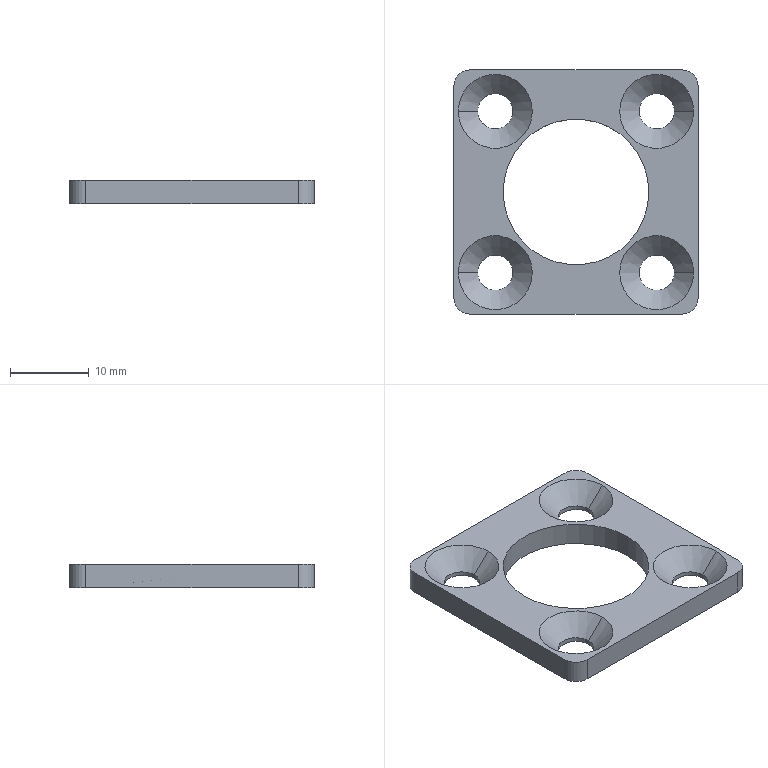Part | NX | features BREP 1 | 1 solid | 28 faces | box 31 x 31 x 3 mm | volume 1644 mm3 | cylinder 14 | cone 8 | plane 6 | commonest cylinder face diameters 4.5 x8 4 x4 18.5 x2
STEP:
#1=CARTESIAN_POINT('',(5.55,10.25,3.));
#2=VERTEX_POINT('',#1);
#3=CARTESIAN_POINT('',(8.,10.25,0.55));
#4=VERTEX_POINT('',#3);
#5=CARTESIAN_POINT('',(5.55,10.25,3.));
#6=DIRECTION('',(-0.7071,0.,0.7071));
#7=VECTOR('',#6,1000.);
#8=LINE('',#5,#7);
#9=EDGE_CURVE('',#2,#4,#8,.F.);
#10=ORIENTED_EDGE('',*,*,#9,.T.);
#11=CARTESIAN_POINT('',(12.5,10.25,0.55));
#12=VERTEX_POINT('',#11);
#13=CARTESIAN_POINT('',(10.25,10.25,0.55));
#14=DIRECTION('',(0.,0.,1.));
#15=DIRECTION('',(1.,0.,0.));
#16=AXIS2_PLACEMENT_3D('',#13,#14,#15);
#17=CIRCLE('',#16,2.25);
#18=EDGE_CURVE('',#12,#4,#17,.T.);
#19=ORIENTED_EDGE('',*,*,#18,.F.);
#20=CARTESIAN_POINT('',(14.95,10.25,3.));
#21=VERTEX_POINT('',#20);
#22=CARTESIAN_POINT('',(14.95,10.25,3.));
#23=DIRECTION('',(0.7071,0.,0.7071));
#24=VECTOR('',#23,1000.);
#25=LINE('',#22,#24);
#26=EDGE_CURVE('',#21,#12,#25,.F.);
#27=ORIENTED_EDGE('',*,*,#26,.F.);
#28=CARTESIAN_POINT('',(10.25,10.25,3.));
#29=DIRECTION('',(0.,0.,1.));
#30=DIRECTION('',(1.,0.,0.));
#31=AXIS2_PLACEMENT_3D('',#28,#29,#30);
#32=CIRCLE('',#31,4.7);
#33=EDGE_CURVE('',#21,#2,#32,.T.);
#34=ORIENTED_EDGE('',*,*,#33,.T.);
#35=EDGE_LOOP('',(#10,#19,#27,#34));
#36=FACE_BOUND('',#35,.T.);
#37=CARTESIAN_POINT('',(10.25,10.25,3.));
#38=DIRECTION('',(0.,0.,1.));
#39=DIRECTION('',(1.,0.,0.));
#40=AXIS2_PLACEMENT_3D('',#37,#38,#39);
#41=CONICAL_SURFACE('',#40,4.7,0.7854);
#42=ADVANCED_FACE('',(#36),#41,.F.);
#43=CARTESIAN_POINT('',(8.,10.25,0.));
#44=VERTEX_POINT('',#43);
#45=CARTESIAN_POINT('',(8.,10.25,3.));
#46=DIRECTION('',(0.,0.,1.));
#47=VECTOR('',#46,1000.);
#48=LINE('',#45,#47);
#49=EDGE_CURVE('',#4,#44,#48,.F.);
#50=ORIENTED_EDGE('',*,*,#49,.T.);
#51=CARTESIAN_POINT('',(12.5,10.25,0.));
#52=VERTEX_POINT('',#51);
#53=CARTESIAN_POINT('',(10.25,10.25,0.));
#54=DIRECTION('',(0.,0.,1.));
#55=DIRECTION('',(1.,0.,0.));
#56=AXIS2_PLACEMENT_3D('',#53,#54,#55);
#57=CIRCLE('',#56,2.25);
#58=EDGE_CURVE('',#52,#44,#57,.T.);
#59=ORIENTED_EDGE('',*,*,#58,.F.);
#60=CARTESIAN_POINT('',(12.5,10.25,3.));
#61=DIRECTION('',(0.,0.,1.));
#62=VECTOR('',#61,1000.);
#63=LINE('',#60,#62);
#64=EDGE_CURVE('',#12,#52,#63,.F.);
#65=ORIENTED_EDGE('',*,*,#64,.F.);
#66=ORIENTED_EDGE('',*,*,#18,.T.);
#67=EDGE_LOOP('',(#50,#59,#65,#66));
#68=FACE_BOUND('',#67,.T.);
#69=CARTESIAN_POINT('',(10.25,10.25,3.));
#70=DIRECTION('',(0.,0.,1.));
#71=DIRECTION('',(1.,0.,0.));
#72=AXIS2_PLACEMENT_3D('',#69,#70,#71);
#73=CYLINDRICAL_SURFACE('',#72,2.25);
#74=ADVANCED_FACE('',(#68),#73,.F.);
#75=CARTESIAN_POINT('',(-14.95,-10.25,3.));
#76=VERTEX_POINT('',#75);
#77=CARTESIAN_POINT('',(-12.5,-10.25,0.55));
#78=VERTEX_POINT('',#77);
#79=CARTESIAN_POINT('',(-14.95,-10.25,3.));
#80=DIRECTION('',(-0.7071,0.,0.7071));
#81=VECTOR('',#80,1000.);
#82=LINE('',#79,#81);
#83=EDGE_CURVE('',#76,#78,#82,.F.);
#84=ORIENTED_EDGE('',*,*,#83,.T.);
#85=CARTESIAN_POINT('',(-8.,-10.25,0.55));
#86=VERTEX_POINT('',#85);
#87=CARTESIAN_POINT('',(-10.25,-10.25,0.55));
#88=DIRECTION('',(0.,0.,1.));
#89=DIRECTION('',(1.,0.,0.));
#90=AXIS2_PLACEMENT_3D('',#87,#88,#89);
#91=CIRCLE('',#90,2.25);
#92=EDGE_CURVE('',#86,#78,#91,.T.);
#93=ORIENTED_EDGE('',*,*,#92,.F.);
#94=CARTESIAN_POINT('',(-5.55,-10.25,3.));
#95=VERTEX_POINT('',#94);
#96=CARTESIAN_POINT('',(-5.55,-10.25,3.));
#97=DIRECTION('',(0.7071,0.,0.7071));
#98=VECTOR('',#97,1000.);
#99=LINE('',#96,#98);
#100=EDGE_CURVE('',#95,#86,#99,.F.);
#101=ORIENTED_EDGE('',*,*,#100,.F.);
#102=CARTESIAN_POINT('',(-10.25,-10.25,3.));
#103=DIRECTION('',(0.,0.,1.));
#104=DIRECTION('',(1.,0.,0.));
#105=AXIS2_PLACEMENT_3D('',#102,#103,#104);
#106=CIRCLE('',#105,4.7);
#107=EDGE_CURVE('',#95,#76,#106,.T.);
#108=ORIENTED_EDGE('',*,*,#107,.T.);
#109=EDGE_LOOP('',(#84,#93,#101,#108));
#110=FACE_BOUND('',#109,.T.);
#111=CARTESIAN_POINT('',(-10.25,-10.25,3.));
#112=DIRECTION('',(0.,0.,1.));
#113=DIRECTION('',(1.,0.,0.));
#114=AXIS2_PLACEMENT_3D('',#111,#112,#113);
#115=CONICAL_SURFACE('',#114,4.7,0.7854);
#116=ADVANCED_FACE('',(#110),#115,.F.);
#117=CARTESIAN_POINT('',(-12.5,-10.25,0.));
#118=VERTEX_POINT('',#117);
#119=CARTESIAN_POINT('',(-12.5,-10.25,3.));
#120=DIRECTION('',(0.,0.,1.));
#121=VECTOR('',#120,1000.);
#122=LINE('',#119,#121);
#123=EDGE_CURVE('',#78,#118,#122,.F.);
#124=ORIENTED_EDGE('',*,*,#123,.T.);
#125=CARTESIAN_POINT('',(-8.,-10.25,0.));
#126=VERTEX_POINT('',#125);
#127=CARTESIAN_POINT('',(-10.25,-10.25,0.));
#128=DIRECTION('',(0.,0.,1.));
#129=DIRECTION('',(1.,0.,0.));
#130=AXIS2_PLACEMENT_3D('',#127,#128,#129);
#131=CIRCLE('',#130,2.25);
#132=EDGE_CURVE('',#126,#118,#131,.T.);
#133=ORIENTED_EDGE('',*,*,#132,.F.);
#134=CARTESIAN_POINT('',(-8.,-10.25,3.));
#135=DIRECTION('',(0.,0.,1.));
#136=VECTOR('',#135,1000.);
#137=LINE('',#134,#136);
#138=EDGE_CURVE('',#86,#126,#137,.F.);
#139=ORIENTED_EDGE('',*,*,#138,.F.);
#140=ORIENTED_EDGE('',*,*,#92,.T.);
#141=EDGE_LOOP('',(#124,#133,#139,#140));
#142=FACE_BOUND('',#141,.T.);
#143=CARTESIAN_POINT('',(-10.25,-10.25,3.));
#144=DIRECTION('',(0.,0.,1.));
#145=DIRECTION('',(1.,0.,0.));
#146=AXIS2_PLACEMENT_3D('',#143,#144,#145);
#147=CYLINDRICAL_SURFACE('',#146,2.25);
#148=ADVANCED_FACE('',(#142),#147,.F.);
#149=CARTESIAN_POINT('',(-14.95,10.25,3.));
#150=VERTEX_POINT('',#149);
#151=CARTESIAN_POINT('',(-12.5,10.25,0.55));
#152=VERTEX_POINT('',#151);
#153=CARTESIAN_POINT('',(-14.95,10.25,3.));
#154=DIRECTION('',(-0.7071,0.,0.7071));
#155=VECTOR('',#154,1000.);
#156=LINE('',#153,#155);
#157=EDGE_CURVE('',#150,#152,#156,.F.);
#158=ORIENTED_EDGE('',*,*,#157,.T.);
#159=CARTESIAN_POINT('',(-8.,10.25,0.55));
#160=VERTEX_POINT('',#159);
#161=CARTESIAN_POINT('',(-10.25,10.25,0.55));
#162=DIRECTION('',(0.,0.,1.));
#163=DIRECTION('',(1.,0.,0.));
#164=AXIS2_PLACEMENT_3D('',#161,#162,#163);
#165=CIRCLE('',#164,2.25);
#166=EDGE_CURVE('',#160,#152,#165,.T.);
#167=ORIENTED_EDGE('',*,*,#166,.F.);
#168=CARTESIAN_POINT('',(-5.55,10.25,3.));
#169=VERTEX_POINT('',#168);
#170=CARTESIAN_POINT('',(-5.55,10.25,3.));
#171=DIRECTION('',(0.7071,0.,0.7071));
#172=VECTOR('',#171,1000.);
#173=LINE('',#170,#172);
#174=EDGE_CURVE('',#169,#160,#173,.F.);
#175=ORIENTED_EDGE('',*,*,#174,.F.);
#176=CARTESIAN_POINT('',(-10.25,10.25,3.));
#177=DIRECTION('',(0.,0.,1.));
#178=DIRECTION('',(1.,0.,0.));
#179=AXIS2_PLACEMENT_3D('',#176,#177,#178);
#180=CIRCLE('',#179,4.7);
#181=EDGE_CURVE('',#169,#150,#180,.T.);
#182=ORIENTED_EDGE('',*,*,#181,.T.);
#183=EDGE_LOOP('',(#158,#167,#175,#182));
#184=FACE_BOUND('',#183,.T.);
#185=CARTESIAN_POINT('',(-10.25,10.25,3.));
#186=DIRECTION('',(0.,0.,1.));
#187=DIRECTION('',(1.,0.,0.));
#188=AXIS2_PLACEMENT_3D('',#185,#186,#187);
#189=CONICAL_SURFACE('',#188,4.7,0.7854);
#190=ADVANCED_FACE('',(#184),#189,.F.);
#191=CARTESIAN_POINT('',(-12.5,10.25,0.));
#192=VERTEX_POINT('',#191);
#193=CARTESIAN_POINT('',(-12.5,10.25,3.));
#194=DIRECTION('',(0.,0.,1.));
#195=VECTOR('',#194,1000.);
#196=LINE('',#193,#195);
#197=EDGE_CURVE('',#152,#192,#196,.F.);
#198=ORIENTED_EDGE('',*,*,#197,.T.);
#199=CARTESIAN_POINT('',(-8.,10.25,0.));
#200=VERTEX_POINT('',#199);
#201=CARTESIAN_POINT('',(-10.25,10.25,0.));
#202=DIRECTION('',(0.,0.,1.));
#203=DIRECTION('',(1.,0.,0.));
#204=AXIS2_PLACEMENT_3D('',#201,#202,#203);
#205=CIRCLE('',#204,2.25);
#206=EDGE_CURVE('',#200,#192,#205,.T.);
#207=ORIENTED_EDGE('',*,*,#206,.F.);
#208=CARTESIAN_POINT('',(-8.,10.25,3.));
#209=DIRECTION('',(0.,0.,1.));
#210=VECTOR('',#209,1000.);
#211=LINE('',#208,#210);
#212=EDGE_CURVE('',#160,#200,#211,.F.);
#213=ORIENTED_EDGE('',*,*,#212,.F.);
#214=ORIENTED_EDGE('',*,*,#166,.T.);
#215=EDGE_LOOP('',(#198,#207,#213,#214));
#216=FACE_BOUND('',#215,.T.);
#217=CARTESIAN_POINT('',(-10.25,10.25,3.));
#218=DIRECTION('',(0.,0.,1.));
#219=DIRECTION('',(1.,0.,0.));
#220=AXIS2_PLACEMENT_3D('',#217,#218,#219);
#221=CYLINDRICAL_SURFACE('',#220,2.25);
#222=ADVANCED_FACE('',(#216),#221,.F.);
#223=CARTESIAN_POINT('',(5.55,-10.25,3.));
#224=VERTEX_POINT('',#223);
#225=CARTESIAN_POINT('',(8.,-10.25,0.55));
#226=VERTEX_POINT('',#225);
#227=CARTESIAN_POINT('',(5.55,-10.25,3.));
#228=DIRECTION('',(-0.7071,0.,0.7071));
#229=VECTOR('',#228,1000.);
#230=LINE('',#227,#229);
#231=EDGE_CURVE('',#224,#226,#230,.F.);
#232=ORIENTED_EDGE('',*,*,#231,.T.);
#233=CARTESIAN_POINT('',(12.5,-10.25,0.55));
#234=VERTEX_POINT('',#233);
#235=CARTESIAN_POINT('',(10.25,-10.25,0.55));
#236=DIRECTION('',(0.,0.,1.));
#237=DIRECTION('',(1.,0.,0.));
#238=AXIS2_PLACEMENT_3D('',#235,#236,#237);
#239=CIRCLE('',#238,2.25);
#240=EDGE_CURVE('',#234,#226,#239,.T.);
#241=ORIENTED_EDGE('',*,*,#240,.F.);
#242=CARTESIAN_POINT('',(14.95,-10.25,3.));
#243=VERTEX_POINT('',#242);
#244=CARTESIAN_POINT('',(14.95,-10.25,3.));
#245=DIRECTION('',(0.7071,0.,0.7071));
#246=VECTOR('',#245,1000.);
#247=LINE('',#244,#246);
#248=EDGE_CURVE('',#243,#234,#247,.F.);
#249=ORIENTED_EDGE('',*,*,#248,.F.);
#250=CARTESIAN_POINT('',(10.25,-10.25,3.));
#251=DIRECTION('',(0.,0.,1.));
#252=DIRECTION('',(1.,0.,0.));
#253=AXIS2_PLACEMENT_3D('',#250,#251,#252);
#254=CIRCLE('',#253,4.7);
#255=EDGE_CURVE('',#243,#224,#254,.T.);
#256=ORIENTED_EDGE('',*,*,#255,.T.);
#257=EDGE_LOOP('',(#232,#241,#249,#256));
#258=FACE_BOUND('',#257,.T.);
#259=CARTESIAN_POINT('',(10.25,-10.25,3.));
#260=DIRECTION('',(0.,0.,1.));
#261=DIRECTION('',(1.,0.,0.));
#262=AXIS2_PLACEMENT_3D('',#259,#260,#261);
#263=CONICAL_SURFACE('',#262,4.7,0.7854);
#264=ADVANCED_FACE('',(#258),#263,.F.);
#265=CARTESIAN_POINT('',(8.,-10.25,0.));
#266=VERTEX_POINT('',#265);
#267=CARTESIAN_POINT('',(8.,-10.25,3.));
#268=DIRECTION('',(0.,0.,1.));
#269=VECTOR('',#268,1000.);
#270=LINE('',#267,#269);
#271=EDGE_CURVE('',#226,#266,#270,.F.);
#272=ORIENTED_EDGE('',*,*,#271,.T.);
#273=CARTESIAN_POINT('',(12.5,-10.25,0.));
#274=VERTEX_POINT('',#273);
#275=CARTESIAN_POINT('',(10.25,-10.25,0.));
#276=DIRECTION('',(0.,0.,1.));
#277=DIRECTION('',(1.,0.,0.));
#278=AXIS2_PLACEMENT_3D('',#275,#276,#277);
#279=CIRCLE('',#278,2.25);
#280=EDGE_CURVE('',#274,#266,#279,.T.);
#281=ORIENTED_EDGE('',*,*,#280,.F.);
#282=CARTESIAN_POINT('',(12.5,-10.25,3.));
#283=DIRECTION('',(0.,0.,1.));
#284=VECTOR('',#283,1000.);
#285=LINE('',#282,#284);
#286=EDGE_CURVE('',#234,#274,#285,.F.);
#287=ORIENTED_EDGE('',*,*,#286,.F.);
#288=ORIENTED_EDGE('',*,*,#240,.T.);
#289=EDGE_LOOP('',(#272,#281,#287,#288));
#290=FACE_BOUND('',#289,.T.);
#291=CARTESIAN_POINT('',(10.25,-10.25,3.));
#292=DIRECTION('',(0.,0.,1.));
#293=DIRECTION('',(1.,0.,0.));
#294=AXIS2_PLACEMENT_3D('',#291,#292,#293);
#295=CYLINDRICAL_SURFACE('',#294,2.25);
#296=ADVANCED_FACE('',(#290),#295,.F.);
#297=CARTESIAN_POINT('',(9.25,0.,3.));
#298=VERTEX_POINT('',#297);
#299=CARTESIAN_POINT('',(9.25,0.,0.));
#300=VERTEX_POINT('',#299);
#301=CARTESIAN_POINT('',(9.25,0.,3.));
#302=DIRECTION('',(0.,0.,-1.));
#303=VECTOR('',#302,1000.);
#304=LINE('',#301,#303);
#305=EDGE_CURVE('',#298,#300,#304,.T.);
#306=ORIENTED_EDGE('',*,*,#305,.F.);
#307=CARTESIAN_POINT('',(-9.25,0.,3.));
#308=VERTEX_POINT('',#307);
#309=CARTESIAN_POINT('',(0.,0.,3.));
#310=DIRECTION('',(0.,0.,1.));
#311=DIRECTION('',(1.,0.,0.));
#312=AXIS2_PLACEMENT_3D('',#309,#310,#311);
#313=CIRCLE('',#312,9.25);
#314=EDGE_CURVE('',#298,#308,#313,.T.);
#315=ORIENTED_EDGE('',*,*,#314,.T.);
#316=CARTESIAN_POINT('',(-9.25,0.,0.));
#317=VERTEX_POINT('',#316);
#318=CARTESIAN_POINT('',(-9.25,0.,3.));
#319=DIRECTION('',(0.,0.,-1.));
#320=VECTOR('',#319,1000.);
#321=LINE('',#318,#320);
#322=EDGE_CURVE('',#308,#317,#321,.T.);
#323=ORIENTED_EDGE('',*,*,#322,.T.);
#324=CARTESIAN_POINT('',(0.,0.,0.));
#325=DIRECTION('',(0.,0.,1.));
#326=DIRECTION('',(1.,0.,0.));
#327=AXIS2_PLACEMENT_3D('',#324,#325,#326);
#328=CIRCLE('',#327,9.25);
#329=EDGE_CURVE('',#300,#317,#328,.T.);
#330=ORIENTED_EDGE('',*,*,#329,.F.);
#331=EDGE_LOOP('',(#306,#315,#323,#330));
#332=FACE_BOUND('',#331,.T.);
#333=CARTESIAN_POINT('',(0.,0.,3.));
#334=DIRECTION('',(0.,0.,-1.));
#335=DIRECTION('',(-1.,0.,0.));
#336=AXIS2_PLACEMENT_3D('',#333,#334,#335);
#337=CYLINDRICAL_SURFACE('',#336,9.25);
#338=ADVANCED_FACE('',(#332),#337,.F.);
#339=CARTESIAN_POINT('',(15.5,-13.5,0.));
#340=VERTEX_POINT('',#339);
#341=CARTESIAN_POINT('',(15.5,13.5,0.));
#342=VERTEX_POINT('',#341);
#343=CARTESIAN_POINT('',(15.5,-13.5,0.));
#344=DIRECTION('',(0.,1.,0.));
#345=VECTOR('',#344,1000.);
#346=LINE('',#343,#345);
#347=EDGE_CURVE('',#340,#342,#346,.T.);
#348=ORIENTED_EDGE('',*,*,#347,.T.);
#349=CARTESIAN_POINT('',(15.5,13.5,3.));
#350=VERTEX_POINT('',#349);
#351=CARTESIAN_POINT('',(15.5,13.5,3.));
#352=DIRECTION('',(0.,0.,-1.));
#353=VECTOR('',#352,1000.);
#354=LINE('',#351,#353);
#355=EDGE_CURVE('',#350,#342,#354,.T.);
#356=ORIENTED_EDGE('',*,*,#355,.F.);
#357=CARTESIAN_POINT('',(15.5,-13.5,3.));
#358=VERTEX_POINT('',#357);
#359=CARTESIAN_POINT('',(15.5,-13.5,3.));
#360=DIRECTION('',(0.,1.,0.));
#361=VECTOR('',#360,1000.);
#362=LINE('',#359,#361);
#363=EDGE_CURVE('',#358,#350,#362,.T.);
#364=ORIENTED_EDGE('',*,*,#363,.F.);
#365=CARTESIAN_POINT('',(15.5,-13.5,3.));
#366=DIRECTION('',(0.,0.,-1.));
#367=VECTOR('',#366,1000.);
#368=LINE('',#365,#367);
#369=EDGE_CURVE('',#358,#340,#368,.T.);
#370=ORIENTED_EDGE('',*,*,#369,.T.);
#371=EDGE_LOOP('',(#348,#356,#364,#370));
#372=FACE_BOUND('',#371,.T.);
#373=CARTESIAN_POINT('',(15.5,-13.5,3.));
#374=DIRECTION('',(-1.,0.,0.));
#375=DIRECTION('',(0.,-1.,0.));
#376=AXIS2_PLACEMENT_3D('',#373,#374,#375);
#377=PLANE('',#376);
#378=ADVANCED_FACE('',(#372),#377,.F.);
#379=CARTESIAN_POINT('',(13.5,-15.5,0.));
#380=VERTEX_POINT('',#379);
#381=CARTESIAN_POINT('',(13.5,-13.5,0.));
#382=DIRECTION('',(0.,0.,1.));
#383=DIRECTION('',(1.,0.,0.));
#384=AXIS2_PLACEMENT_3D('',#381,#382,#383);
#385=CIRCLE('',#384,2.);
#386=EDGE_CURVE('',#380,#340,#385,.T.);
#387=ORIENTED_EDGE('',*,*,#386,.T.);
#388=ORIENTED_EDGE('',*,*,#369,.F.);
#389=CARTESIAN_POINT('',(13.5,-15.5,3.));
#390=VERTEX_POINT('',#389);
#391=CARTESIAN_POINT('',(13.5,-13.5,3.));
#392=DIRECTION('',(0.,0.,1.));
#393=DIRECTION('',(1.,0.,0.));
#394=AXIS2_PLACEMENT_3D('',#391,#392,#393);
#395=CIRCLE('',#394,2.);
#396=EDGE_CURVE('',#390,#358,#395,.T.);
#397=ORIENTED_EDGE('',*,*,#396,.F.);
#398=CARTESIAN_POINT('',(13.5,-15.5,3.));
#399=DIRECTION('',(0.,0.,-1.));
#400=VECTOR('',#399,1000.);
#401=LINE('',#398,#400);
#402=EDGE_CURVE('',#390,#380,#401,.T.);
#403=ORIENTED_EDGE('',*,*,#402,.T.);
#404=EDGE_LOOP('',(#387,#388,#397,#403));
#405=FACE_BOUND('',#404,.T.);
#406=CARTESIAN_POINT('',(13.5,-13.5,3.));
#407=DIRECTION('',(0.,0.,-1.));
#408=DIRECTION('',(-1.,0.,0.));
#409=AXIS2_PLACEMENT_3D('',#406,#407,#408);
#410=CYLINDRICAL_SURFACE('',#409,2.);
#411=ADVANCED_FACE('',(#405),#410,.T.);
#412=CARTESIAN_POINT('',(-13.5,-15.5,0.));
#413=VERTEX_POINT('',#412);
#414=CARTESIAN_POINT('',(-13.5,-15.5,0.));
#415=DIRECTION('',(1.,0.,0.));
#416=VECTOR('',#415,1000.);
#417=LINE('',#414,#416);
#418=EDGE_CURVE('',#413,#380,#417,.T.);
#419=ORIENTED_EDGE('',*,*,#418,.T.);
#420=ORIENTED_EDGE('',*,*,#402,.F.);
#421=CARTESIAN_POINT('',(-13.5,-15.5,3.));
#422=VERTEX_POINT('',#421);
#423=CARTESIAN_POINT('',(-13.5,-15.5,3.));
#424=DIRECTION('',(1.,0.,0.));
#425=VECTOR('',#424,1000.);
#426=LINE('',#423,#425);
#427=EDGE_CURVE('',#422,#390,#426,.T.);
#428=ORIENTED_EDGE('',*,*,#427,.F.);
#429=CARTESIAN_POINT('',(-13.5,-15.5,3.));
#430=DIRECTION('',(0.,0.,-1.));
#431=VECTOR('',#430,1000.);
#432=LINE('',#429,#431);
#433=EDGE_CURVE('',#422,#413,#432,.T.);
#434=ORIENTED_EDGE('',*,*,#433,.T.);
#435=EDGE_LOOP('',(#419,#420,#428,#434));
#436=FACE_BOUND('',#435,.T.);
#437=CARTESIAN_POINT('',(-13.5,-15.5,3.));
#438=DIRECTION('',(0.,1.,0.));
#439=DIRECTION('',(0.,0.,1.));
#440=AXIS2_PLACEMENT_3D('',#437,#438,#439);
#441=PLANE('',#440);
#442=ADVANCED_FACE('',(#436),#441,.F.);
#443=CARTESIAN_POINT('',(-15.5,-13.5,0.));
#444=VERTEX_POINT('',#443);
#445=CARTESIAN_POINT('',(-13.5,-13.5,0.));
#446=DIRECTION('',(0.,0.,1.));
#447=DIRECTION('',(-1.,0.,0.));
#448=AXIS2_PLACEMENT_3D('',#445,#446,#447);
#449=CIRCLE('',#448,2.);
#450=EDGE_CURVE('',#444,#413,#449,.T.);
#451=ORIENTED_EDGE('',*,*,#450,.T.);
#452=ORIENTED_EDGE('',*,*,#433,.F.);
#453=CARTESIAN_POINT('',(-15.5,-13.5,3.));
#454=VERTEX_POINT('',#453);
#455=CARTESIAN_POINT('',(-13.5,-13.5,3.));
#456=DIRECTION('',(0.,0.,1.));
#457=DIRECTION('',(-1.,0.,0.));
#458=AXIS2_PLACEMENT_3D('',#455,#456,#457);
#459=CIRCLE('',#458,2.);
#460=EDGE_CURVE('',#454,#422,#459,.T.);
#461=ORIENTED_EDGE('',*,*,#460,.F.);
#462=CARTESIAN_POINT('',(-15.5,-13.5,3.));
#463=DIRECTION('',(0.,0.,-1.));
#464=VECTOR('',#463,1000.);
#465=LINE('',#462,#464);
#466=EDGE_CURVE('',#454,#444,#465,.T.);
#467=ORIENTED_EDGE('',*,*,#466,.T.);
#468=EDGE_LOOP('',(#451,#452,#461,#467));
#469=FACE_BOUND('',#468,.T.);
#470=CARTESIAN_POINT('',(-13.5,-13.5,3.));
#471=DIRECTION('',(0.,0.,-1.));
#472=DIRECTION('',(-1.,0.,0.));
#473=AXIS2_PLACEMENT_3D('',#470,#471,#472);
#474=CYLINDRICAL_SURFACE('',#473,2.);
#475=ADVANCED_FACE('',(#469),#474,.T.);
#476=CARTESIAN_POINT('',(-15.5,13.5,0.));
#477=VERTEX_POINT('',#476);
#478=CARTESIAN_POINT('',(-15.5,-13.5,0.));
#479=DIRECTION('',(0.,-1.,0.));
#480=VECTOR('',#479,1000.);
#481=LINE('',#478,#480);
#482=EDGE_CURVE('',#477,#444,#481,.T.);
#483=ORIENTED_EDGE('',*,*,#482,.T.);
#484=ORIENTED_EDGE('',*,*,#466,.F.);
#485=CARTESIAN_POINT('',(-15.5,13.5,3.));
#486=VERTEX_POINT('',#485);
#487=CARTESIAN_POINT('',(-15.5,-13.5,3.));
#488=DIRECTION('',(0.,-1.,0.));
#489=VECTOR('',#488,1000.);
#490=LINE('',#487,#489);
#491=EDGE_CURVE('',#486,#454,#490,.T.);
#492=ORIENTED_EDGE('',*,*,#491,.F.);
#493=CARTESIAN_POINT('',(-15.5,13.5,3.));
#494=DIRECTION('',(0.,0.,-1.));
#495=VECTOR('',#494,1000.);
#496=LINE('',#493,#495);
#497=EDGE_CURVE('',#486,#477,#496,.T.);
#498=ORIENTED_EDGE('',*,*,#497,.T.);
#499=EDGE_LOOP('',(#483,#484,#492,#498));
#500=FACE_BOUND('',#499,.T.);
#501=CARTESIAN_POINT('',(-15.5,-13.5,3.));
#502=DIRECTION('',(1.,0.,0.));
#503=DIRECTION('',(0.,1.,0.));
#504=AXIS2_PLACEMENT_3D('',#501,#502,#503);
#505=PLANE('',#504);
#506=ADVANCED_FACE('',(#500),#505,.F.);
#507=CARTESIAN_POINT('',(-13.5,15.5,0.));
#508=VERTEX_POINT('',#507);
#509=CARTESIAN_POINT('',(-13.5,13.5,0.));
#510=DIRECTION('',(0.,0.,1.));
#511=DIRECTION('',(-1.,0.,0.));
#512=AXIS2_PLACEMENT_3D('',#509,#510,#511);
#513=CIRCLE('',#512,2.);
#514=EDGE_CURVE('',#508,#477,#513,.T.);
#515=ORIENTED_EDGE('',*,*,#514,.T.);
#516=ORIENTED_EDGE('',*,*,#497,.F.);
#517=CARTESIAN_POINT('',(-13.5,15.5,3.));
#518=VERTEX_POINT('',#517);
#519=CARTESIAN_POINT('',(-13.5,13.5,3.));
#520=DIRECTION('',(0.,0.,1.));
#521=DIRECTION('',(-1.,0.,0.));
#522=AXIS2_PLACEMENT_3D('',#519,#520,#521);
#523=CIRCLE('',#522,2.);
#524=EDGE_CURVE('',#518,#486,#523,.T.);
#525=ORIENTED_EDGE('',*,*,#524,.F.);
#526=CARTESIAN_POINT('',(-13.5,15.5,3.));
#527=DIRECTION('',(0.,0.,-1.));
#528=VECTOR('',#527,1000.);
#529=LINE('',#526,#528);
#530=EDGE_CURVE('',#518,#508,#529,.T.);
#531=ORIENTED_EDGE('',*,*,#530,.T.);
#532=EDGE_LOOP('',(#515,#516,#525,#531));
#533=FACE_BOUND('',#532,.T.);
#534=CARTESIAN_POINT('',(-13.5,13.5,3.));
#535=DIRECTION('',(0.,0.,-1.));
#536=DIRECTION('',(-1.,0.,0.));
#537=AXIS2_PLACEMENT_3D('',#534,#535,#536);
#538=CYLINDRICAL_SURFACE('',#537,2.);
#539=ADVANCED_FACE('',(#533),#538,.T.);
#540=CARTESIAN_POINT('',(13.5,15.5,0.));
#541=VERTEX_POINT('',#540);
#542=CARTESIAN_POINT('',(-13.5,15.5,0.));
#543=DIRECTION('',(-1.,0.,0.));
#544=VECTOR('',#543,1000.);
#545=LINE('',#542,#544);
#546=EDGE_CURVE('',#541,#508,#545,.T.);
#547=ORIENTED_EDGE('',*,*,#546,.T.);
#548=ORIENTED_EDGE('',*,*,#530,.F.);
#549=CARTESIAN_POINT('',(13.5,15.5,3.));
#550=VERTEX_POINT('',#549);
#551=CARTESIAN_POINT('',(-13.5,15.5,3.));
#552=DIRECTION('',(-1.,0.,0.));
#553=VECTOR('',#552,1000.);
#554=LINE('',#551,#553);
#555=EDGE_CURVE('',#550,#518,#554,.T.);
#556=ORIENTED_EDGE('',*,*,#555,.F.);
#557=CARTESIAN_POINT('',(13.5,15.5,3.));
#558=DIRECTION('',(0.,0.,-1.));
#559=VECTOR('',#558,1000.);
#560=LINE('',#557,#559);
#561=EDGE_CURVE('',#550,#541,#560,.T.);
#562=ORIENTED_EDGE('',*,*,#561,.T.);
#563=EDGE_LOOP('',(#547,#548,#556,#562));
#564=FACE_BOUND('',#563,.T.);
#565=CARTESIAN_POINT('',(-13.5,15.5,3.));
#566=DIRECTION('',(0.,-1.,0.));
#567=DIRECTION('',(0.,0.,-1.));
#568=AXIS2_PLACEMENT_3D('',#565,#566,#567);
#569=PLANE('',#568);
#570=ADVANCED_FACE('',(#564),#569,.F.);
#571=CARTESIAN_POINT('',(13.5,13.5,0.));
#572=DIRECTION('',(0.,0.,1.));
#573=DIRECTION('',(1.,0.,0.));
#574=AXIS2_PLACEMENT_3D('',#571,#572,#573);
#575=CIRCLE('',#574,2.);
#576=EDGE_CURVE('',#342,#541,#575,.T.);
#577=ORIENTED_EDGE('',*,*,#576,.T.);
#578=ORIENTED_EDGE('',*,*,#561,.F.);
#579=CARTESIAN_POINT('',(13.5,13.5,3.));
#580=DIRECTION('',(0.,0.,1.));
#581=DIRECTION('',(1.,0.,0.));
#582=AXIS2_PLACEMENT_3D('',#579,#580,#581);
#583=CIRCLE('',#582,2.);
#584=EDGE_CURVE('',#350,#550,#583,.T.);
#585=ORIENTED_EDGE('',*,*,#584,.F.);
#586=ORIENTED_EDGE('',*,*,#355,.T.);
#587=EDGE_LOOP('',(#577,#578,#585,#586));
#588=FACE_BOUND('',#587,.T.);
#589=CARTESIAN_POINT('',(13.5,13.5,3.));
#590=DIRECTION('',(0.,0.,-1.));
#591=DIRECTION('',(-1.,0.,0.));
#592=AXIS2_PLACEMENT_3D('',#589,#590,#591);
#593=CYLINDRICAL_SURFACE('',#592,2.);
#594=ADVANCED_FACE('',(#588),#593,.T.);
#595=CARTESIAN_POINT('',(0.,0.,0.));
#596=DIRECTION('',(0.,0.,1.));
#597=DIRECTION('',(1.,0.,0.));
#598=AXIS2_PLACEMENT_3D('',#595,#596,#597);
#599=CIRCLE('',#598,9.25);
#600=EDGE_CURVE('',#317,#300,#599,.T.);
#601=ORIENTED_EDGE('',*,*,#600,.T.);
#602=ORIENTED_EDGE('',*,*,#329,.T.);
#603=EDGE_LOOP('',(#601,#602));
#604=FACE_BOUND('',#603,.T.);
#605=ORIENTED_EDGE('',*,*,#576,.F.);
#606=ORIENTED_EDGE('',*,*,#347,.F.);
#607=ORIENTED_EDGE('',*,*,#386,.F.);
#608=ORIENTED_EDGE('',*,*,#418,.F.);
#609=ORIENTED_EDGE('',*,*,#450,.F.);
#610=ORIENTED_EDGE('',*,*,#482,.F.);
#611=ORIENTED_EDGE('',*,*,#514,.F.);
#612=ORIENTED_EDGE('',*,*,#546,.F.);
#613=EDGE_LOOP('',(#605,#606,#607,#608,#609,#610,#611,#612));
#614=FACE_BOUND('',#613,.T.);
#615=ORIENTED_EDGE('',*,*,#280,.T.);
#616=CARTESIAN_POINT('',(10.25,-10.25,0.));
#617=DIRECTION('',(0.,0.,1.));
#618=DIRECTION('',(1.,0.,0.));
#619=AXIS2_PLACEMENT_3D('',#616,#617,#618);
#620=CIRCLE('',#619,2.25);
#621=EDGE_CURVE('',#266,#274,#620,.T.);
#622=ORIENTED_EDGE('',*,*,#621,.T.);
#623=EDGE_LOOP('',(#615,#622));
#624=FACE_BOUND('',#623,.T.);
#625=ORIENTED_EDGE('',*,*,#206,.T.);
#626=CARTESIAN_POINT('',(-10.25,10.25,0.));
#627=DIRECTION('',(0.,0.,1.));
#628=DIRECTION('',(1.,0.,0.));
#629=AXIS2_PLACEMENT_3D('',#626,#627,#628);
#630=CIRCLE('',#629,2.25);
#631=EDGE_CURVE('',#192,#200,#630,.T.);
#632=ORIENTED_EDGE('',*,*,#631,.T.);
#633=EDGE_LOOP('',(#625,#632));
#634=FACE_BOUND('',#633,.T.);
#635=ORIENTED_EDGE('',*,*,#132,.T.);
#636=CARTESIAN_POINT('',(-10.25,-10.25,0.));
#637=DIRECTION('',(0.,0.,1.));
#638=DIRECTION('',(1.,0.,0.));
#639=AXIS2_PLACEMENT_3D('',#636,#637,#638);
#640=CIRCLE('',#639,2.25);
#641=EDGE_CURVE('',#118,#126,#640,.T.);
#642=ORIENTED_EDGE('',*,*,#641,.T.);
#643=EDGE_LOOP('',(#635,#642));
#644=FACE_BOUND('',#643,.T.);
#645=ORIENTED_EDGE('',*,*,#58,.T.);
#646=CARTESIAN_POINT('',(10.25,10.25,0.));
#647=DIRECTION('',(0.,0.,1.));
#648=DIRECTION('',(1.,0.,0.));
#649=AXIS2_PLACEMENT_3D('',#646,#647,#648);
#650=CIRCLE('',#649,2.25);
#651=EDGE_CURVE('',#44,#52,#650,.T.);
#652=ORIENTED_EDGE('',*,*,#651,.T.);
#653=EDGE_LOOP('',(#645,#652));
#654=FACE_BOUND('',#653,.T.);
#655=CARTESIAN_POINT('',(13.5,13.5,0.));
#656=DIRECTION('',(0.,0.,1.));
#657=DIRECTION('',(1.,0.,0.));
#658=AXIS2_PLACEMENT_3D('',#655,#656,#657);
#659=PLANE('',#658);
#660=ADVANCED_FACE('',(#604,#614,#624,#634,#644,#654),#659,.F.);
#661=CARTESIAN_POINT('',(0.,0.,3.));
#662=DIRECTION('',(0.,0.,1.));
#663=DIRECTION('',(1.,0.,0.));
#664=AXIS2_PLACEMENT_3D('',#661,#662,#663);
#665=CIRCLE('',#664,9.25);
#666=EDGE_CURVE('',#308,#298,#665,.T.);
#667=ORIENTED_EDGE('',*,*,#666,.F.);
#668=ORIENTED_EDGE('',*,*,#314,.F.);
#669=EDGE_LOOP('',(#667,#668));
#670=FACE_BOUND('',#669,.T.);
#671=ORIENTED_EDGE('',*,*,#584,.T.);
#672=ORIENTED_EDGE('',*,*,#555,.T.);
#673=ORIENTED_EDGE('',*,*,#524,.T.);
#674=ORIENTED_EDGE('',*,*,#491,.T.);
#675=ORIENTED_EDGE('',*,*,#460,.T.);
#676=ORIENTED_EDGE('',*,*,#427,.T.);
#677=ORIENTED_EDGE('',*,*,#396,.T.);
#678=ORIENTED_EDGE('',*,*,#363,.T.);
#679=EDGE_LOOP('',(#671,#672,#673,#674,#675,#676,#677,#678));
#680=FACE_BOUND('',#679,.T.);
#681=ORIENTED_EDGE('',*,*,#255,.F.);
#682=CARTESIAN_POINT('',(10.25,-10.25,3.));
#683=DIRECTION('',(0.,0.,1.));
#684=DIRECTION('',(1.,0.,0.));
#685=AXIS2_PLACEMENT_3D('',#682,#683,#684);
#686=CIRCLE('',#685,4.7);
#687=EDGE_CURVE('',#224,#243,#686,.T.);
#688=ORIENTED_EDGE('',*,*,#687,.F.);
#689=EDGE_LOOP('',(#681,#688));
#690=FACE_BOUND('',#689,.T.);
#691=ORIENTED_EDGE('',*,*,#181,.F.);
#692=CARTESIAN_POINT('',(-10.25,10.25,3.));
#693=DIRECTION('',(0.,0.,1.));
#694=DIRECTION('',(1.,0.,0.));
#695=AXIS2_PLACEMENT_3D('',#692,#693,#694);
#696=CIRCLE('',#695,4.7);
#697=EDGE_CURVE('',#150,#169,#696,.T.);
#698=ORIENTED_EDGE('',*,*,#697,.F.);
#699=EDGE_LOOP('',(#691,#698));
#700=FACE_BOUND('',#699,.T.);
#701=ORIENTED_EDGE('',*,*,#107,.F.);
#702=CARTESIAN_POINT('',(-10.25,-10.25,3.));
#703=DIRECTION('',(0.,0.,1.));
#704=DIRECTION('',(1.,0.,0.));
#705=AXIS2_PLACEMENT_3D('',#702,#703,#704);
#706=CIRCLE('',#705,4.7);
#707=EDGE_CURVE('',#76,#95,#706,.T.);
#708=ORIENTED_EDGE('',*,*,#707,.F.);
#709=EDGE_LOOP('',(#701,#708));
#710=FACE_BOUND('',#709,.T.);
#711=ORIENTED_EDGE('',*,*,#33,.F.);
#712=CARTESIAN_POINT('',(10.25,10.25,3.));
#713=DIRECTION('',(0.,0.,1.));
#714=DIRECTION('',(1.,0.,0.));
#715=AXIS2_PLACEMENT_3D('',#712,#713,#714);
#716=CIRCLE('',#715,4.7);
#717=EDGE_CURVE('',#2,#21,#716,.T.);
#718=ORIENTED_EDGE('',*,*,#717,.F.);
#719=EDGE_LOOP('',(#711,#718));
#720=FACE_BOUND('',#719,.T.);
#721=CARTESIAN_POINT('',(13.5,13.5,3.));
#722=DIRECTION('',(0.,0.,1.));
#723=DIRECTION('',(1.,0.,0.));
#724=AXIS2_PLACEMENT_3D('',#721,#722,#723);
#725=PLANE('',#724);
#726=ADVANCED_FACE('',(#670,#680,#690,#700,#710,#720),#725,.T.);
#727=ORIENTED_EDGE('',*,*,#666,.T.);
#728=ORIENTED_EDGE('',*,*,#305,.T.);
#729=ORIENTED_EDGE('',*,*,#600,.F.);
#730=ORIENTED_EDGE('',*,*,#322,.F.);
#731=EDGE_LOOP('',(#727,#728,#729,#730));
#732=FACE_BOUND('',#731,.T.);
#733=CARTESIAN_POINT('',(0.,0.,3.));
#734=DIRECTION('',(0.,0.,-1.));
#735=DIRECTION('',(-1.,0.,0.));
#736=AXIS2_PLACEMENT_3D('',#733,#734,#735);
#737=CYLINDRICAL_SURFACE('',#736,9.25);
#738=ADVANCED_FACE('',(#732),#737,.F.);
#739=ORIENTED_EDGE('',*,*,#621,.F.);
#740=ORIENTED_EDGE('',*,*,#271,.F.);
#741=CARTESIAN_POINT('',(10.25,-10.25,0.55));
#742=DIRECTION('',(0.,0.,1.));
#743=DIRECTION('',(1.,0.,0.));
#744=AXIS2_PLACEMENT_3D('',#741,#742,#743);
#745=CIRCLE('',#744,2.25);
#746=EDGE_CURVE('',#226,#234,#745,.T.);
#747=ORIENTED_EDGE('',*,*,#746,.T.);
#748=ORIENTED_EDGE('',*,*,#286,.T.);
#749=EDGE_LOOP('',(#739,#740,#747,#748));
#750=FACE_BOUND('',#749,.T.);
#751=CARTESIAN_POINT('',(10.25,-10.25,3.));
#752=DIRECTION('',(0.,0.,1.));
#753=DIRECTION('',(1.,0.,0.));
#754=AXIS2_PLACEMENT_3D('',#751,#752,#753);
#755=CYLINDRICAL_SURFACE('',#754,2.25);
#756=ADVANCED_FACE('',(#750),#755,.F.);
#757=ORIENTED_EDGE('',*,*,#746,.F.);
#758=ORIENTED_EDGE('',*,*,#231,.F.);
#759=ORIENTED_EDGE('',*,*,#687,.T.);
#760=ORIENTED_EDGE('',*,*,#248,.T.);
#761=EDGE_LOOP('',(#757,#758,#759,#760));
#762=FACE_BOUND('',#761,.T.);
#763=CARTESIAN_POINT('',(10.25,-10.25,3.));
#764=DIRECTION('',(0.,0.,1.));
#765=DIRECTION('',(1.,0.,0.));
#766=AXIS2_PLACEMENT_3D('',#763,#764,#765);
#767=CONICAL_SURFACE('',#766,4.7,0.7854);
#768=ADVANCED_FACE('',(#762),#767,.F.);
#769=ORIENTED_EDGE('',*,*,#631,.F.);
#770=ORIENTED_EDGE('',*,*,#197,.F.);
#771=CARTESIAN_POINT('',(-10.25,10.25,0.55));
#772=DIRECTION('',(0.,0.,1.));
#773=DIRECTION('',(1.,0.,0.));
#774=AXIS2_PLACEMENT_3D('',#771,#772,#773);
#775=CIRCLE('',#774,2.25);
#776=EDGE_CURVE('',#152,#160,#775,.T.);
#777=ORIENTED_EDGE('',*,*,#776,.T.);
#778=ORIENTED_EDGE('',*,*,#212,.T.);
#779=EDGE_LOOP('',(#769,#770,#777,#778));
#780=FACE_BOUND('',#779,.T.);
#781=CARTESIAN_POINT('',(-10.25,10.25,3.));
#782=DIRECTION('',(0.,0.,1.));
#783=DIRECTION('',(1.,0.,0.));
#784=AXIS2_PLACEMENT_3D('',#781,#782,#783);
#785=CYLINDRICAL_SURFACE('',#784,2.25);
#786=ADVANCED_FACE('',(#780),#785,.F.);
#787=ORIENTED_EDGE('',*,*,#776,.F.);
#788=ORIENTED_EDGE('',*,*,#157,.F.);
#789=ORIENTED_EDGE('',*,*,#697,.T.);
#790=ORIENTED_EDGE('',*,*,#174,.T.);
#791=EDGE_LOOP('',(#787,#788,#789,#790));
#792=FACE_BOUND('',#791,.T.);
#793=CARTESIAN_POINT('',(-10.25,10.25,3.));
#794=DIRECTION('',(0.,0.,1.));
#795=DIRECTION('',(1.,0.,0.));
#796=AXIS2_PLACEMENT_3D('',#793,#794,#795);
#797=CONICAL_SURFACE('',#796,4.7,0.7854);
#798=ADVANCED_FACE('',(#792),#797,.F.);
#799=ORIENTED_EDGE('',*,*,#641,.F.);
#800=ORIENTED_EDGE('',*,*,#123,.F.);
#801=CARTESIAN_POINT('',(-10.25,-10.25,0.55));
#802=DIRECTION('',(0.,0.,1.));
#803=DIRECTION('',(1.,0.,0.));
#804=AXIS2_PLACEMENT_3D('',#801,#802,#803);
#805=CIRCLE('',#804,2.25);
#806=EDGE_CURVE('',#78,#86,#805,.T.);
#807=ORIENTED_EDGE('',*,*,#806,.T.);
#808=ORIENTED_EDGE('',*,*,#138,.T.);
#809=EDGE_LOOP('',(#799,#800,#807,#808));
#810=FACE_BOUND('',#809,.T.);
#811=CARTESIAN_POINT('',(-10.25,-10.25,3.));
#812=DIRECTION('',(0.,0.,1.));
#813=DIRECTION('',(1.,0.,0.));
#814=AXIS2_PLACEMENT_3D('',#811,#812,#813);
#815=CYLINDRICAL_SURFACE('',#814,2.25);
#816=ADVANCED_FACE('',(#810),#815,.F.);
#817=ORIENTED_EDGE('',*,*,#806,.F.);
#818=ORIENTED_EDGE('',*,*,#83,.F.);
#819=ORIENTED_EDGE('',*,*,#707,.T.);
#820=ORIENTED_EDGE('',*,*,#100,.T.);
#821=EDGE_LOOP('',(#817,#818,#819,#820));
#822=FACE_BOUND('',#821,.T.);
#823=CARTESIAN_POINT('',(-10.25,-10.25,3.));
#824=DIRECTION('',(0.,0.,1.));
#825=DIRECTION('',(1.,0.,0.));
#826=AXIS2_PLACEMENT_3D('',#823,#824,#825);
#827=CONICAL_SURFACE('',#826,4.7,0.7854);
#828=ADVANCED_FACE('',(#822),#827,.F.);
#829=ORIENTED_EDGE('',*,*,#651,.F.);
#830=ORIENTED_EDGE('',*,*,#49,.F.);
#831=CARTESIAN_POINT('',(10.25,10.25,0.55));
#832=DIRECTION('',(0.,0.,1.));
#833=DIRECTION('',(1.,0.,0.));
#834=AXIS2_PLACEMENT_3D('',#831,#832,#833);
#835=CIRCLE('',#834,2.25);
#836=EDGE_CURVE('',#4,#12,#835,.T.);
#837=ORIENTED_EDGE('',*,*,#836,.T.);
#838=ORIENTED_EDGE('',*,*,#64,.T.);
#839=EDGE_LOOP('',(#829,#830,#837,#838));
#840=FACE_BOUND('',#839,.T.);
#841=CARTESIAN_POINT('',(10.25,10.25,3.));
#842=DIRECTION('',(0.,0.,1.));
#843=DIRECTION('',(1.,0.,0.));
#844=AXIS2_PLACEMENT_3D('',#841,#842,#843);
#845=CYLINDRICAL_SURFACE('',#844,2.25);
#846=ADVANCED_FACE('',(#840),#845,.F.);
#847=ORIENTED_EDGE('',*,*,#836,.F.);
#848=ORIENTED_EDGE('',*,*,#9,.F.);
#849=ORIENTED_EDGE('',*,*,#717,.T.);
#850=ORIENTED_EDGE('',*,*,#26,.T.);
#851=EDGE_LOOP('',(#847,#848,#849,#850));
#852=FACE_BOUND('',#851,.T.);
#853=CARTESIAN_POINT('',(10.25,10.25,3.));
#854=DIRECTION('',(0.,0.,1.));
#855=DIRECTION('',(1.,0.,0.));
#856=AXIS2_PLACEMENT_3D('',#853,#854,#855);
#857=CONICAL_SURFACE('',#856,4.7,0.7854);
#858=ADVANCED_FACE('',(#852),#857,.F.);
#859=CLOSED_SHELL('',(#42,#74,#116,#148,#190,#222,#264,#296,#338,#378,#411,#442,#475,#506,#539,#570,#594,#660,#726,#738,#756,#768,#786,#798,#816,#828,#846,#858));
#860=MANIFOLD_SOLID_BREP('',#859);
#861=(LENGTH_UNIT()NAMED_UNIT(*)SI_UNIT(.MILLI.,.METRE.));
#862=UNCERTAINTY_MEASURE_WITH_UNIT(LENGTH_MEASURE(0.00001),#861,'','');
#863=(NAMED_UNIT(*)PLANE_ANGLE_UNIT()SI_UNIT($,.RADIAN.));
#864=(NAMED_UNIT(*)SI_UNIT($,.STERADIAN.)SOLID_ANGLE_UNIT());
#865=(GEOMETRIC_REPRESENTATION_CONTEXT(3)GLOBAL_UNCERTAINTY_ASSIGNED_CONTEXT((#862))GLOBAL_UNIT_ASSIGNED_CONTEXT((#861,#863,#864))REPRESENTATION_CONTEXT('',''));
#866=ADVANCED_BREP_SHAPE_REPRESENTATION('',(#860),#865);